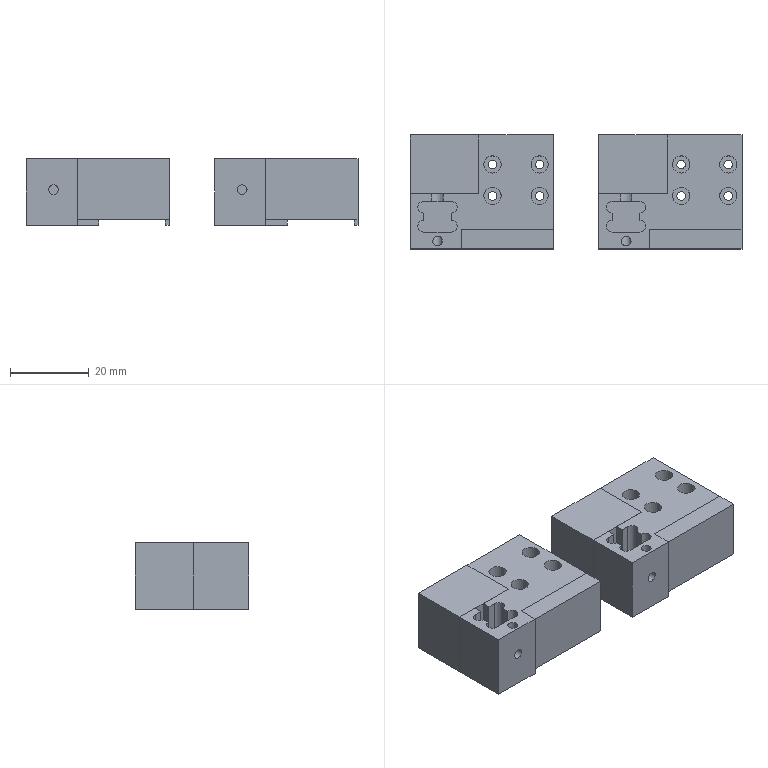NC program | NX | posted with a generic post | part box 84.5 x 29 x 17 mm
Whole program:
N10 G17 G21 G94 G90
(DRILLING_COPY_1_COPY , TOOL : D6A45)
N12 T07 M6
N14 G54
N16 G17 G0 G90 X0.6 Y11.25 B0. C0. S5000 M3
N18 G43 Z30. H7
N20 G94 G81 G98 Z-1.35 F250. R3.
N22 G80
N24 G0 X0.6 Y11.25 Z30.
N26 M5
(DRILLING_COPY_COPY_1 , TOOL : 2.5ZT)
N28 T12 M6
N30 G54
N32 G17 G0 G90 X0.6 Y11.25 B0. C0. S2000 M3
N34 G43 Z30. H12
N36 G94 G83 G98 Z-6.551 F120. Q2. R3.
N38 G80
N40 G0 X0.6 Y11.25 Z30.
N42 M5
(FLOOR_WALL_1_1_COPY , TOOL : D10)
N44 T10 M6
N46 G54
N48 G17 G0 G90 X16.5 Y-23.25 B0. C0. S9500 M3
N50 G43 Z30. H10
N52 Z-1.9
N54 G94 G1 Z-4.9 F1000.
N56 X13.5
N58 X-13.5 F2500.
N60 Y-22.753
N62 X13.5
N64 Y-22.256
N66 X-13.5
N68 Y-21.76
N70 X13.5
N72 Y-21.263
N74 X-13.5
N76 Y-20.766
N78 X13.5
N80 Y-20.269
N82 X-13.5
N84 Y-19.772
N86 X13.5
N88 Y-19.276
N90 X-13.5
N92 Y-18.779
N94 X13.5
N96 Y-18.282
N98 X-13.5
N100 Y-17.785
N102 X13.5
N104 Y-17.288
N106 X-13.5
N108 Y-16.791
N110 X13.5
N112 Y-16.295
N114 X-13.5
N116 Y-15.798
N118 X13.5
N120 Y-15.301
N122 X-13.5
N124 Y-14.804
N126 X13.5
N128 Y-14.307
N130 X-13.5
N132 Y-13.811
N134 X13.5
N136 Y-13.314
N138 X-13.5
N140 Y-12.817
N142 X13.5
N144 Y-12.32
N146 X-13.5
N148 Y-12.25
N150 X-12. Y-11.823
N152 X13.5
N154 Y-11.327
N156 X-12.
N158 Y-10.83
N160 X13.5
N162 Y-10.333
N164 X-12.
N166 Y-9.836
N168 X13.5
N170 Y-9.339
N172 X-12.
N174 Y-8.843
N176 X13.5
N178 Y-8.346
N180 X-12.
N182 Y-7.849
N184 X13.5
N186 Y-7.352
N188 X-12.
N190 Y-6.855
N192 X13.5
N194 Y-6.359
N196 X-12.
N198 Y-5.862
N200 X13.5
N202 Y-5.365
N204 X-12.
N206 X-13.5 Y-5.25
N208 Y-4.868
N210 X13.5
N212 Y-4.371
N214 X-13.5
N216 Y-3.874
N218 X13.5
N220 Y-3.378
N222 X-13.5
N224 Y-2.881
N226 X13.5
N228 Y-2.384
N230 X-13.5
N232 Y-1.887
N234 X13.5
N236 Y-1.39
N238 X-13.5
N240 Y-0.894
N242 X13.5
N244 Y-0.397
N246 X-13.5
N248 Y0.1
N250 X13.5
N252 X16.65
N254 Z-1.9
N256 G0 Z30.
N258 M5
N260 M2